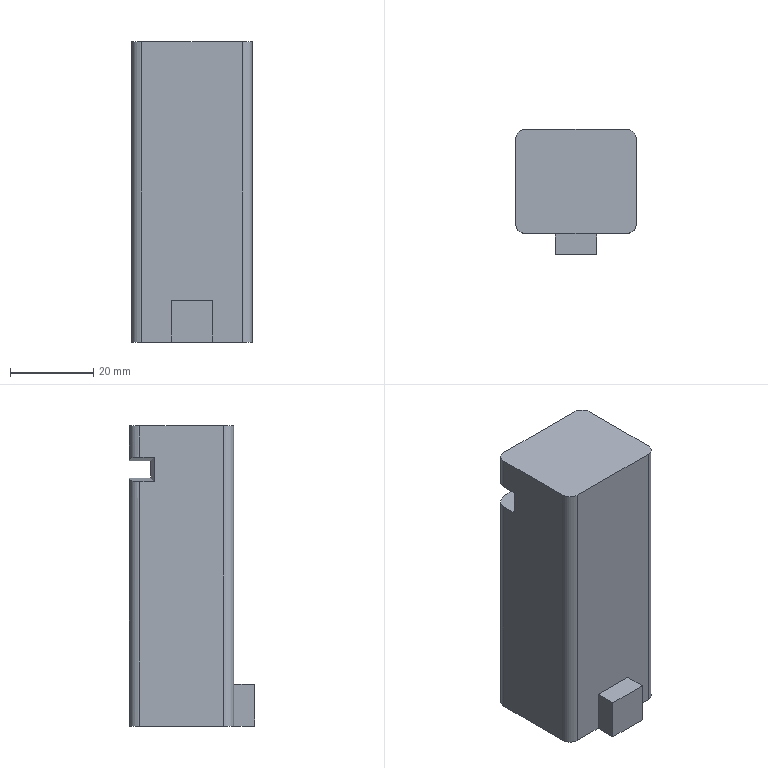Part | NX | features 1605340631 2 | 1 solid | 28 faces | box 29 x 30 x 72 mm | volume 45526 mm3 | plane 21 | cylinder 7 | commonest cylinder face diameters 5 x6 17 x1
STEP:
#1=CARTESIAN_POINT('',(-139.5,-95.3,2.1));
#2=VERTEX_POINT('',#1);
#3=CARTESIAN_POINT('',(-120.5,-95.3,2.1));
#4=VERTEX_POINT('',#3);
#5=CARTESIAN_POINT('',(-131.872,-95.3,2.1));
#6=DIRECTION('',(1.,0.,0.));
#7=VECTOR('',#6,1000.);
#8=LINE('',#5,#7);
#9=EDGE_CURVE('',#2,#4,#8,.T.);
#10=ORIENTED_EDGE('',*,*,#9,.T.);
#11=CARTESIAN_POINT('',(-120.5,-95.3,-2.));
#12=VERTEX_POINT('',#11);
#13=CARTESIAN_POINT('',(-120.5,-95.3,-0.1));
#14=DIRECTION('',(0.,0.,-1.));
#15=VECTOR('',#14,1000.);
#16=LINE('',#13,#15);
#17=EDGE_CURVE('',#4,#12,#16,.T.);
#18=ORIENTED_EDGE('',*,*,#17,.T.);
#19=CARTESIAN_POINT('',(-139.5,-95.3,-2.));
#20=VERTEX_POINT('',#19);
#21=CARTESIAN_POINT('',(165.,-95.3,-2.));
#22=DIRECTION('',(-1.,0.,0.));
#23=VECTOR('',#22,1000.);
#24=LINE('',#21,#23);
#25=EDGE_CURVE('',#12,#20,#24,.T.);
#26=ORIENTED_EDGE('',*,*,#25,.T.);
#27=CARTESIAN_POINT('',(-139.5,-95.3,-0.1));
#28=DIRECTION('',(0.,0.,1.));
#29=VECTOR('',#28,1000.);
#30=LINE('',#27,#29);
#31=EDGE_CURVE('',#20,#2,#30,.T.);
#32=ORIENTED_EDGE('',*,*,#31,.T.);
#33=EDGE_LOOP('',(#10,#18,#26,#32));
#34=FACE_BOUND('',#33,.T.);
#35=CARTESIAN_POINT('',(-131.872,-95.3,-0.1));
#36=DIRECTION('',(0.,1.,0.));
#37=DIRECTION('',(-1.,0.,0.));
#38=AXIS2_PLACEMENT_3D('',#35,#36,#37);
#39=PLANE('',#38);
#40=ADVANCED_FACE('',(#34),#39,.T.);
#41=ORIENTED_EDGE('',*,*,#25,.F.);
#42=CARTESIAN_POINT('',(-120.5,-90.2,-2.));
#43=VERTEX_POINT('',#42);
#44=CARTESIAN_POINT('',(-120.5,-31.936,-2.));
#45=DIRECTION('',(0.,1.,0.));
#46=VECTOR('',#45,1000.);
#47=LINE('',#44,#46);
#48=EDGE_CURVE('',#12,#43,#47,.T.);
#49=ORIENTED_EDGE('',*,*,#48,.T.);
#50=CARTESIAN_POINT('',(-139.5,-90.2,-2.));
#51=VERTEX_POINT('',#50);
#52=CARTESIAN_POINT('',(165.,-90.2,-2.));
#53=DIRECTION('',(-1.,0.,0.));
#54=VECTOR('',#53,1000.);
#55=LINE('',#52,#54);
#56=EDGE_CURVE('',#43,#51,#55,.T.);
#57=ORIENTED_EDGE('',*,*,#56,.T.);
#58=CARTESIAN_POINT('',(-139.5,-31.936,-2.));
#59=DIRECTION('',(0.,-1.,0.));
#60=VECTOR('',#59,1000.);
#61=LINE('',#58,#60);
#62=EDGE_CURVE('',#51,#20,#61,.T.);
#63=ORIENTED_EDGE('',*,*,#62,.T.);
#64=EDGE_LOOP('',(#41,#49,#57,#63));
#65=FACE_BOUND('',#64,.T.);
#66=CARTESIAN_POINT('',(165.,-31.936,-2.));
#67=DIRECTION('',(0.,0.,1.));
#68=DIRECTION('',(1.,0.,0.));
#69=AXIS2_PLACEMENT_3D('',#66,#67,#68);
#70=PLANE('',#69);
#71=ADVANCED_FACE('',(#65),#70,.T.);
#72=ORIENTED_EDGE('',*,*,#56,.F.);
#73=CARTESIAN_POINT('',(-118.,-90.2,-2.441));
#74=VERTEX_POINT('',#73);
#75=CARTESIAN_POINT('',(-133.512,-90.2,0.2944));
#76=DIRECTION('',(-0.9848,0.,0.1736));
#77=VECTOR('',#76,1000.);
#78=LINE('',#75,#77);
#79=EDGE_CURVE('',#43,#74,#78,.F.);
#80=ORIENTED_EDGE('',*,*,#79,.T.);
#81=CARTESIAN_POINT('',(-118.,-90.2,-61.5));
#82=VERTEX_POINT('',#81);
#83=CARTESIAN_POINT('',(-118.,-90.2,-36.501));
#84=DIRECTION('',(0.,0.,-1.));
#85=VECTOR('',#84,1000.);
#86=LINE('',#83,#85);
#87=EDGE_CURVE('',#74,#82,#86,.T.);
#88=ORIENTED_EDGE('',*,*,#87,.T.);
#89=CARTESIAN_POINT('',(-142.,-90.2,-61.5));
#90=VERTEX_POINT('',#89);
#91=CARTESIAN_POINT('',(-180.,-90.2,-61.5));
#92=DIRECTION('',(1.,0.,0.));
#93=VECTOR('',#92,1000.);
#94=LINE('',#91,#93);
#95=EDGE_CURVE('',#90,#82,#94,.T.);
#96=ORIENTED_EDGE('',*,*,#95,.F.);
#97=CARTESIAN_POINT('',(-142.,-90.2,-2.441));
#98=VERTEX_POINT('',#97);
#99=CARTESIAN_POINT('',(-142.,-90.2,-36.501));
#100=DIRECTION('',(0.,0.,-1.));
#101=VECTOR('',#100,1000.);
#102=LINE('',#99,#101);
#103=EDGE_CURVE('',#90,#98,#102,.F.);
#104=ORIENTED_EDGE('',*,*,#103,.T.);
#105=CARTESIAN_POINT('',(-145.885,-90.2,-3.126));
#106=DIRECTION('',(-0.9848,0.,-0.1736));
#107=VECTOR('',#106,1000.);
#108=LINE('',#105,#107);
#109=EDGE_CURVE('',#98,#51,#108,.F.);
#110=ORIENTED_EDGE('',*,*,#109,.T.);
#111=EDGE_LOOP('',(#72,#80,#88,#96,#104,#110));
#112=FACE_BOUND('',#111,.T.);
#113=CARTESIAN_POINT('',(-140.,-90.2,-36.501));
#114=DIRECTION('',(0.,1.,0.));
#115=DIRECTION('',(0.,0.,1.));
#116=AXIS2_PLACEMENT_3D('',#113,#114,#115);
#117=PLANE('',#116);
#118=ADVANCED_FACE('',(#112),#117,.T.);
#119=CARTESIAN_POINT('',(-139.5,-90.2,2.1));
#120=VERTEX_POINT('',#119);
#121=CARTESIAN_POINT('',(-120.5,-90.2,2.1));
#122=VERTEX_POINT('',#121);
#123=CARTESIAN_POINT('',(-140.,-90.2,2.1));
#124=DIRECTION('',(1.,0.,0.));
#125=VECTOR('',#124,1000.);
#126=LINE('',#123,#125);
#127=EDGE_CURVE('',#120,#122,#126,.T.);
#128=ORIENTED_EDGE('',*,*,#127,.T.);
#129=CARTESIAN_POINT('',(-120.5,-95.3,2.1));
#130=DIRECTION('',(0.,-1.,0.));
#131=VECTOR('',#130,1000.);
#132=LINE('',#129,#131);
#133=EDGE_CURVE('',#122,#4,#132,.T.);
#134=ORIENTED_EDGE('',*,*,#133,.T.);
#135=ORIENTED_EDGE('',*,*,#9,.F.);
#136=CARTESIAN_POINT('',(-139.5,-92.2,2.1));
#137=DIRECTION('',(0.,1.,0.));
#138=VECTOR('',#137,1000.);
#139=LINE('',#136,#138);
#140=EDGE_CURVE('',#2,#120,#139,.T.);
#141=ORIENTED_EDGE('',*,*,#140,.T.);
#142=EDGE_LOOP('',(#128,#134,#135,#141));
#143=FACE_BOUND('',#142,.T.);
#144=CARTESIAN_POINT('',(-140.,-110.2,2.1));
#145=DIRECTION('',(0.,0.,1.));
#146=DIRECTION('',(1.,0.,0.));
#147=AXIS2_PLACEMENT_3D('',#144,#145,#146);
#148=PLANE('',#147);
#149=ADVANCED_FACE('',(#143),#148,.F.);
#150=CARTESIAN_POINT('',(-118.,-90.2,10.5));
#151=VERTEX_POINT('',#150);
#152=CARTESIAN_POINT('',(-118.,-90.2,2.541));
#153=VERTEX_POINT('',#152);
#154=CARTESIAN_POINT('',(-118.,-90.2,-37.901));
#155=DIRECTION('',(0.,0.,1.));
#156=VECTOR('',#155,1000.);
#157=LINE('',#154,#156);
#158=EDGE_CURVE('',#151,#153,#157,.F.);
#159=ORIENTED_EDGE('',*,*,#158,.T.);
#160=CARTESIAN_POINT('',(-146.253,-90.2,-2.441));
#161=DIRECTION('',(-0.9848,0.,-0.1736));
#162=VECTOR('',#161,1000.);
#163=LINE('',#160,#162);
#164=EDGE_CURVE('',#153,#122,#163,.T.);
#165=ORIENTED_EDGE('',*,*,#164,.T.);
#166=ORIENTED_EDGE('',*,*,#127,.F.);
#167=CARTESIAN_POINT('',(-142.,-90.2,2.541));
#168=VERTEX_POINT('',#167);
#169=CARTESIAN_POINT('',(-133.144,-90.2,0.9793));
#170=DIRECTION('',(-0.9848,0.,0.1736));
#171=VECTOR('',#170,1000.);
#172=LINE('',#169,#171);
#173=EDGE_CURVE('',#120,#168,#172,.T.);
#174=ORIENTED_EDGE('',*,*,#173,.T.);
#175=CARTESIAN_POINT('',(-142.,-90.2,10.5));
#176=VERTEX_POINT('',#175);
#177=CARTESIAN_POINT('',(-142.,-90.2,-37.901));
#178=DIRECTION('',(0.,0.,1.));
#179=VECTOR('',#178,1000.);
#180=LINE('',#177,#179);
#181=EDGE_CURVE('',#168,#176,#180,.T.);
#182=ORIENTED_EDGE('',*,*,#181,.T.);
#183=CARTESIAN_POINT('',(-140.,-90.2,10.5));
#184=DIRECTION('',(-1.,0.,0.));
#185=VECTOR('',#184,1000.);
#186=LINE('',#183,#185);
#187=EDGE_CURVE('',#151,#176,#186,.T.);
#188=ORIENTED_EDGE('',*,*,#187,.F.);
#189=EDGE_LOOP('',(#159,#165,#166,#174,#182,#188));
#190=FACE_BOUND('',#189,.T.);
#191=CARTESIAN_POINT('',(-140.,-90.2,-37.901));
#192=DIRECTION('',(0.,1.,0.));
#193=DIRECTION('',(0.,0.,1.));
#194=AXIS2_PLACEMENT_3D('',#191,#192,#193);
#195=PLANE('',#194);
#196=ADVANCED_FACE('',(#190),#195,.T.);
#197=CARTESIAN_POINT('',(-142.,-115.2,10.5));
#198=VERTEX_POINT('',#197);
#199=CARTESIAN_POINT('',(-118.,-115.2,10.5));
#200=VERTEX_POINT('',#199);
#201=CARTESIAN_POINT('',(-120.,-115.2,10.5));
#202=DIRECTION('',(1.,0.,0.));
#203=VECTOR('',#202,1000.);
#204=LINE('',#201,#203);
#205=EDGE_CURVE('',#198,#200,#204,.T.);
#206=ORIENTED_EDGE('',*,*,#205,.F.);
#207=CARTESIAN_POINT('',(-142.,-115.2,-61.5));
#208=VERTEX_POINT('',#207);
#209=CARTESIAN_POINT('',(-142.,-115.2,-36.501));
#210=DIRECTION('',(0.,0.,-1.));
#211=VECTOR('',#210,1000.);
#212=LINE('',#209,#211);
#213=EDGE_CURVE('',#198,#208,#212,.T.);
#214=ORIENTED_EDGE('',*,*,#213,.T.);
#215=CARTESIAN_POINT('',(-135.,-115.2,-61.5));
#216=VERTEX_POINT('',#215);
#217=CARTESIAN_POINT('',(-180.,-115.2,-61.5));
#218=DIRECTION('',(-1.,0.,0.));
#219=VECTOR('',#218,1000.);
#220=LINE('',#217,#219);
#221=EDGE_CURVE('',#216,#208,#220,.T.);
#222=ORIENTED_EDGE('',*,*,#221,.F.);
#223=CARTESIAN_POINT('',(-135.,-115.2,-51.5));
#224=VERTEX_POINT('',#223);
#225=CARTESIAN_POINT('',(-135.,-115.2,-26.501));
#226=DIRECTION('',(0.,0.,-1.));
#227=VECTOR('',#226,1000.);
#228=LINE('',#225,#227);
#229=EDGE_CURVE('',#224,#216,#228,.T.);
#230=ORIENTED_EDGE('',*,*,#229,.F.);
#231=CARTESIAN_POINT('',(-125.,-115.2,-51.5));
#232=VERTEX_POINT('',#231);
#233=CARTESIAN_POINT('',(-120.,-115.2,-51.5));
#234=DIRECTION('',(1.,0.,0.));
#235=VECTOR('',#234,1000.);
#236=LINE('',#233,#235);
#237=EDGE_CURVE('',#224,#232,#236,.T.);
#238=ORIENTED_EDGE('',*,*,#237,.T.);
#239=CARTESIAN_POINT('',(-125.,-115.2,-61.5));
#240=VERTEX_POINT('',#239);
#241=CARTESIAN_POINT('',(-125.,-115.2,-26.501));
#242=DIRECTION('',(0.,0.,-1.));
#243=VECTOR('',#242,1000.);
#244=LINE('',#241,#243);
#245=EDGE_CURVE('',#232,#240,#244,.T.);
#246=ORIENTED_EDGE('',*,*,#245,.T.);
#247=CARTESIAN_POINT('',(-118.,-115.2,-61.5));
#248=VERTEX_POINT('',#247);
#249=CARTESIAN_POINT('',(-180.,-115.2,-61.5));
#250=DIRECTION('',(-1.,0.,0.));
#251=VECTOR('',#250,1000.);
#252=LINE('',#249,#251);
#253=EDGE_CURVE('',#248,#240,#252,.T.);
#254=ORIENTED_EDGE('',*,*,#253,.F.);
#255=CARTESIAN_POINT('',(-118.,-115.2,-36.501));
#256=DIRECTION('',(0.,0.,-1.));
#257=VECTOR('',#256,1000.);
#258=LINE('',#255,#257);
#259=EDGE_CURVE('',#248,#200,#258,.F.);
#260=ORIENTED_EDGE('',*,*,#259,.T.);
#261=EDGE_LOOP('',(#206,#214,#222,#230,#238,#246,#254,#260));
#262=FACE_BOUND('',#261,.T.);
#263=CARTESIAN_POINT('',(-120.,-115.2,-36.501));
#264=DIRECTION('',(0.,-1.,0.));
#265=DIRECTION('',(0.,0.,-1.));
#266=AXIS2_PLACEMENT_3D('',#263,#264,#265);
#267=PLANE('',#266);
#268=ADVANCED_FACE('',(#262),#267,.T.);
#269=CARTESIAN_POINT('',(-138.5,-102.7,-61.5));
#270=VERTEX_POINT('',#269);
#271=CARTESIAN_POINT('',(-130.,-102.7,-61.5));
#272=DIRECTION('',(0.,0.,-1.));
#273=DIRECTION('',(-1.,0.,0.));
#274=AXIS2_PLACEMENT_3D('',#271,#272,#273);
#275=CIRCLE('',#274,8.5);
#276=EDGE_CURVE('',#270,#270,#275,.F.);
#277=ORIENTED_EDGE('',*,*,#276,.T.);
#278=EDGE_LOOP('',(#277));
#279=FACE_BOUND('',#278,.T.);
#280=ORIENTED_EDGE('',*,*,#253,.T.);
#281=CARTESIAN_POINT('',(-125.,-120.2,-61.5));
#282=VERTEX_POINT('',#281);
#283=CARTESIAN_POINT('',(-125.,-167.2,-61.5));
#284=DIRECTION('',(0.,1.,0.));
#285=VECTOR('',#284,1000.);
#286=LINE('',#283,#285);
#287=EDGE_CURVE('',#282,#240,#286,.T.);
#288=ORIENTED_EDGE('',*,*,#287,.F.);
#289=CARTESIAN_POINT('',(-135.,-120.2,-61.5));
#290=VERTEX_POINT('',#289);
#291=CARTESIAN_POINT('',(-180.,-120.2,-61.5));
#292=DIRECTION('',(-1.,0.,0.));
#293=VECTOR('',#292,1000.);
#294=LINE('',#291,#293);
#295=EDGE_CURVE('',#282,#290,#294,.T.);
#296=ORIENTED_EDGE('',*,*,#295,.T.);
#297=CARTESIAN_POINT('',(-135.,-167.2,-61.5));
#298=DIRECTION('',(0.,1.,0.));
#299=VECTOR('',#298,1000.);
#300=LINE('',#297,#299);
#301=EDGE_CURVE('',#290,#216,#300,.T.);
#302=ORIENTED_EDGE('',*,*,#301,.T.);
#303=ORIENTED_EDGE('',*,*,#221,.T.);
#304=CARTESIAN_POINT('',(-144.5,-112.7,-61.5));
#305=VERTEX_POINT('',#304);
#306=CARTESIAN_POINT('',(-142.,-112.7,-61.5));
#307=DIRECTION('',(0.,0.,-1.));
#308=DIRECTION('',(-1.,0.,0.));
#309=AXIS2_PLACEMENT_3D('',#306,#307,#308);
#310=CIRCLE('',#309,2.5);
#311=EDGE_CURVE('',#208,#305,#310,.T.);
#312=ORIENTED_EDGE('',*,*,#311,.T.);
#313=CARTESIAN_POINT('',(-144.5,-92.7,-61.5));
#314=VERTEX_POINT('',#313);
#315=CARTESIAN_POINT('',(-144.5,-167.2,-61.5));
#316=DIRECTION('',(0.,1.,0.));
#317=VECTOR('',#316,1000.);
#318=LINE('',#315,#317);
#319=EDGE_CURVE('',#305,#314,#318,.T.);
#320=ORIENTED_EDGE('',*,*,#319,.T.);
#321=CARTESIAN_POINT('',(-142.,-92.7,-61.5));
#322=DIRECTION('',(0.,0.,-1.));
#323=DIRECTION('',(-1.,0.,0.));
#324=AXIS2_PLACEMENT_3D('',#321,#322,#323);
#325=CIRCLE('',#324,2.5);
#326=EDGE_CURVE('',#314,#90,#325,.T.);
#327=ORIENTED_EDGE('',*,*,#326,.T.);
#328=ORIENTED_EDGE('',*,*,#95,.T.);
#329=CARTESIAN_POINT('',(-115.5,-92.7,-61.5));
#330=VERTEX_POINT('',#329);
#331=CARTESIAN_POINT('',(-118.,-92.7,-61.5));
#332=DIRECTION('',(0.,0.,-1.));
#333=DIRECTION('',(-1.,0.,0.));
#334=AXIS2_PLACEMENT_3D('',#331,#332,#333);
#335=CIRCLE('',#334,2.5);
#336=EDGE_CURVE('',#82,#330,#335,.T.);
#337=ORIENTED_EDGE('',*,*,#336,.T.);
#338=CARTESIAN_POINT('',(-115.5,-112.7,-61.5));
#339=VERTEX_POINT('',#338);
#340=CARTESIAN_POINT('',(-115.5,-167.2,-61.5));
#341=DIRECTION('',(0.,-1.,0.));
#342=VECTOR('',#341,1000.);
#343=LINE('',#340,#342);
#344=EDGE_CURVE('',#330,#339,#343,.T.);
#345=ORIENTED_EDGE('',*,*,#344,.T.);
#346=CARTESIAN_POINT('',(-118.,-112.7,-61.5));
#347=DIRECTION('',(0.,0.,-1.));
#348=DIRECTION('',(-1.,0.,0.));
#349=AXIS2_PLACEMENT_3D('',#346,#347,#348);
#350=CIRCLE('',#349,2.5);
#351=EDGE_CURVE('',#339,#248,#350,.T.);
#352=ORIENTED_EDGE('',*,*,#351,.T.);
#353=EDGE_LOOP('',(#280,#288,#296,#302,#303,#312,#320,#327,#328,#337,#345,#352));
#354=FACE_BOUND('',#353,.T.);
#355=CARTESIAN_POINT('',(-180.,-167.2,-61.5));
#356=DIRECTION('',(0.,0.,-1.));
#357=DIRECTION('',(-1.,0.,0.));
#358=AXIS2_PLACEMENT_3D('',#355,#356,#357);
#359=PLANE('',#358);
#360=ADVANCED_FACE('',(#279,#354),#359,.T.);
#361=ORIENTED_EDGE('',*,*,#87,.F.);
#362=CARTESIAN_POINT('',(-115.5,-92.7,-2.882));
#363=VERTEX_POINT('',#362);
#364=CARTESIAN_POINT('',(-118.,-92.7,-2.441));
#365=DIRECTION('',(-0.1736,0.,-0.9848));
#366=DIRECTION('',(0.9848,0.,-0.1736));
#367=AXIS2_PLACEMENT_3D('',#364,#365,#366);
#368=ELLIPSE('',#367,2.539,2.5);
#369=EDGE_CURVE('',#74,#363,#368,.T.);
#370=ORIENTED_EDGE('',*,*,#369,.T.);
#371=CARTESIAN_POINT('',(-115.5,-92.7,-36.501));
#372=DIRECTION('',(0.,0.,-1.));
#373=VECTOR('',#372,1000.);
#374=LINE('',#371,#373);
#375=EDGE_CURVE('',#330,#363,#374,.F.);
#376=ORIENTED_EDGE('',*,*,#375,.F.);
#377=ORIENTED_EDGE('',*,*,#336,.F.);
#378=EDGE_LOOP('',(#361,#370,#376,#377));
#379=FACE_BOUND('',#378,.T.);
#380=CARTESIAN_POINT('',(-118.,-92.7,-36.501));
#381=DIRECTION('',(0.,0.,-1.));
#382=DIRECTION('',(-1.,0.,0.));
#383=AXIS2_PLACEMENT_3D('',#380,#381,#382);
#384=CYLINDRICAL_SURFACE('',#383,2.5);
#385=ADVANCED_FACE('',(#379),#384,.T.);
#386=ORIENTED_EDGE('',*,*,#351,.F.);
#387=CARTESIAN_POINT('',(-115.5,-112.7,10.5));
#388=VERTEX_POINT('',#387);
#389=CARTESIAN_POINT('',(-115.5,-112.7,-36.501));
#390=DIRECTION('',(0.,0.,-1.));
#391=VECTOR('',#390,1000.);
#392=LINE('',#389,#391);
#393=EDGE_CURVE('',#388,#339,#392,.T.);
#394=ORIENTED_EDGE('',*,*,#393,.F.);
#395=CARTESIAN_POINT('',(-118.,-112.7,10.5));
#396=DIRECTION('',(0.,0.,1.));
#397=DIRECTION('',(1.,0.,0.));
#398=AXIS2_PLACEMENT_3D('',#395,#396,#397);
#399=CIRCLE('',#398,2.5);
#400=EDGE_CURVE('',#200,#388,#399,.T.);
#401=ORIENTED_EDGE('',*,*,#400,.F.);
#402=ORIENTED_EDGE('',*,*,#259,.F.);
#403=EDGE_LOOP('',(#386,#394,#401,#402));
#404=FACE_BOUND('',#403,.T.);
#405=CARTESIAN_POINT('',(-118.,-112.7,-36.501));
#406=DIRECTION('',(0.,0.,-1.));
#407=DIRECTION('',(-1.,0.,0.));
#408=AXIS2_PLACEMENT_3D('',#405,#406,#407);
#409=CYLINDRICAL_SURFACE('',#408,2.5);
#410=ADVANCED_FACE('',(#404),#409,.T.);
#411=CARTESIAN_POINT('',(-115.5,-96.182,-2.882));
#412=VERTEX_POINT('',#411);
#413=CARTESIAN_POINT('',(-115.5,-96.182,2.982));
#414=VERTEX_POINT('',#413);
#415=CARTESIAN_POINT('',(-115.5,-96.182,-36.501));
#416=DIRECTION('',(0.,0.,1.));
#417=VECTOR('',#416,1000.);
#418=LINE('',#415,#417);
#419=EDGE_CURVE('',#412,#414,#418,.T.);
#420=ORIENTED_EDGE('',*,*,#419,.T.);
#421=CARTESIAN_POINT('',(-115.5,-92.7,2.982));
#422=VERTEX_POINT('',#421);
#423=CARTESIAN_POINT('',(-115.5,-92.2,2.982));
#424=DIRECTION('',(0.,1.,0.));
#425=VECTOR('',#424,1000.);
#426=LINE('',#423,#425);
#427=EDGE_CURVE('',#414,#422,#426,.T.);
#428=ORIENTED_EDGE('',*,*,#427,.T.);
#429=CARTESIAN_POINT('',(-115.5,-92.7,10.5));
#430=VERTEX_POINT('',#429);
#431=CARTESIAN_POINT('',(-115.5,-92.7,-36.501));
#432=DIRECTION('',(0.,0.,1.));
#433=VECTOR('',#432,1000.);
#434=LINE('',#431,#433);
#435=EDGE_CURVE('',#422,#430,#434,.T.);
#436=ORIENTED_EDGE('',*,*,#435,.T.);
#437=CARTESIAN_POINT('',(-115.5,-90.2,10.5));
#438=DIRECTION('',(0.,1.,0.));
#439=VECTOR('',#438,1000.);
#440=LINE('',#437,#439);
#441=EDGE_CURVE('',#388,#430,#440,.T.);
#442=ORIENTED_EDGE('',*,*,#441,.F.);
#443=ORIENTED_EDGE('',*,*,#393,.T.);
#444=ORIENTED_EDGE('',*,*,#344,.F.);
#445=ORIENTED_EDGE('',*,*,#375,.T.);
#446=CARTESIAN_POINT('',(-115.5,-90.2,-2.882));
#447=DIRECTION('',(0.,-1.,0.));
#448=VECTOR('',#447,1000.);
#449=LINE('',#446,#448);
#450=EDGE_CURVE('',#363,#412,#449,.T.);
#451=ORIENTED_EDGE('',*,*,#450,.T.);
#452=EDGE_LOOP('',(#420,#428,#436,#442,#443,#444,#445,#451));
#453=FACE_BOUND('',#452,.T.);
#454=CARTESIAN_POINT('',(-115.5,-90.2,-36.501));
#455=DIRECTION('',(1.,0.,0.));
#456=DIRECTION('',(0.,0.,-1.));
#457=AXIS2_PLACEMENT_3D('',#454,#455,#456);
#458=PLANE('',#457);
#459=ADVANCED_FACE('',(#453),#458,.T.);
#460=ORIENTED_EDGE('',*,*,#435,.F.);
#461=CARTESIAN_POINT('',(-118.,-92.7,2.541));
#462=DIRECTION('',(0.1736,0.,-0.9848));
#463=DIRECTION('',(0.9848,0.,0.1736));
#464=AXIS2_PLACEMENT_3D('',#461,#462,#463);
#465=ELLIPSE('',#464,2.539,2.5);
#466=EDGE_CURVE('',#422,#153,#465,.F.);
#467=ORIENTED_EDGE('',*,*,#466,.T.);
#468=ORIENTED_EDGE('',*,*,#158,.F.);
#469=CARTESIAN_POINT('',(-118.,-92.7,10.5));
#470=DIRECTION('',(0.,0.,1.));
#471=DIRECTION('',(1.,0.,0.));
#472=AXIS2_PLACEMENT_3D('',#469,#470,#471);
#473=CIRCLE('',#472,2.5);
#474=EDGE_CURVE('',#430,#151,#473,.T.);
#475=ORIENTED_EDGE('',*,*,#474,.F.);
#476=EDGE_LOOP('',(#460,#467,#468,#475));
#477=FACE_BOUND('',#476,.T.);
#478=CARTESIAN_POINT('',(-118.,-92.7,-36.501));
#479=DIRECTION('',(0.,0.,1.));
#480=DIRECTION('',(1.,0.,0.));
#481=AXIS2_PLACEMENT_3D('',#478,#479,#480);
#482=CYLINDRICAL_SURFACE('',#481,2.5);
#483=ADVANCED_FACE('',(#477),#482,.T.);
#484=CARTESIAN_POINT('',(-144.5,-92.7,10.5));
#485=VERTEX_POINT('',#484);
#486=CARTESIAN_POINT('',(-144.5,-92.7,2.982));
#487=VERTEX_POINT('',#486);
#488=CARTESIAN_POINT('',(-144.5,-92.7,-36.501));
#489=DIRECTION('',(0.,0.,1.));
#490=VECTOR('',#489,1000.);
#491=LINE('',#488,#490);
#492=EDGE_CURVE('',#485,#487,#491,.F.);
#493=ORIENTED_EDGE('',*,*,#492,.T.);
#494=CARTESIAN_POINT('',(-144.5,-96.182,2.982));
#495=VERTEX_POINT('',#494);
#496=CARTESIAN_POINT('',(-144.5,-95.3,2.982));
#497=DIRECTION('',(0.,-1.,0.));
#498=VECTOR('',#497,1000.);
#499=LINE('',#496,#498);
#500=EDGE_CURVE('',#487,#495,#499,.T.);
#501=ORIENTED_EDGE('',*,*,#500,.T.);
#502=CARTESIAN_POINT('',(-144.5,-96.182,-2.882));
#503=VERTEX_POINT('',#502);
#504=CARTESIAN_POINT('',(-144.5,-96.182,-36.501));
#505=DIRECTION('',(0.,0.,-1.));
#506=VECTOR('',#505,1000.);
#507=LINE('',#504,#506);
#508=EDGE_CURVE('',#495,#503,#507,.T.);
#509=ORIENTED_EDGE('',*,*,#508,.T.);
#510=CARTESIAN_POINT('',(-144.5,-92.7,-2.882));
#511=VERTEX_POINT('',#510);
#512=CARTESIAN_POINT('',(-144.5,-110.2,-2.882));
#513=DIRECTION('',(0.,1.,0.));
#514=VECTOR('',#513,1000.);
#515=LINE('',#512,#514);
#516=EDGE_CURVE('',#503,#511,#515,.T.);
#517=ORIENTED_EDGE('',*,*,#516,.T.);
#518=CARTESIAN_POINT('',(-144.5,-92.7,-36.501));
#519=DIRECTION('',(0.,0.,-1.));
#520=VECTOR('',#519,1000.);
#521=LINE('',#518,#520);
#522=EDGE_CURVE('',#511,#314,#521,.T.);
#523=ORIENTED_EDGE('',*,*,#522,.T.);
#524=ORIENTED_EDGE('',*,*,#319,.F.);
#525=CARTESIAN_POINT('',(-144.5,-112.7,10.5));
#526=VERTEX_POINT('',#525);
#527=CARTESIAN_POINT('',(-144.5,-112.7,-36.501));
#528=DIRECTION('',(0.,0.,-1.));
#529=VECTOR('',#528,1000.);
#530=LINE('',#527,#529);
#531=EDGE_CURVE('',#305,#526,#530,.F.);
#532=ORIENTED_EDGE('',*,*,#531,.T.);
#533=CARTESIAN_POINT('',(-144.5,-110.2,10.5));
#534=DIRECTION('',(0.,-1.,0.));
#535=VECTOR('',#534,1000.);
#536=LINE('',#533,#535);
#537=EDGE_CURVE('',#485,#526,#536,.T.);
#538=ORIENTED_EDGE('',*,*,#537,.F.);
#539=EDGE_LOOP('',(#493,#501,#509,#517,#523,#524,#532,#538));
#540=FACE_BOUND('',#539,.T.);
#541=CARTESIAN_POINT('',(-144.5,-110.2,-36.501));
#542=DIRECTION('',(-1.,0.,0.));
#543=DIRECTION('',(0.,0.,1.));
#544=AXIS2_PLACEMENT_3D('',#541,#542,#543);
#545=PLANE('',#544);
#546=ADVANCED_FACE('',(#540),#545,.T.);
#547=ORIENTED_EDGE('',*,*,#311,.F.);
#548=ORIENTED_EDGE('',*,*,#213,.F.);
#549=CARTESIAN_POINT('',(-142.,-112.7,10.5));
#550=DIRECTION('',(0.,0.,1.));
#551=DIRECTION('',(1.,0.,0.));
#552=AXIS2_PLACEMENT_3D('',#549,#550,#551);
#553=CIRCLE('',#552,2.5);
#554=EDGE_CURVE('',#526,#198,#553,.T.);
#555=ORIENTED_EDGE('',*,*,#554,.F.);
#556=ORIENTED_EDGE('',*,*,#531,.F.);
#557=EDGE_LOOP('',(#547,#548,#555,#556));
#558=FACE_BOUND('',#557,.T.);
#559=CARTESIAN_POINT('',(-142.,-112.7,-36.501));
#560=DIRECTION('',(0.,0.,-1.));
#561=DIRECTION('',(-1.,0.,0.));
#562=AXIS2_PLACEMENT_3D('',#559,#560,#561);
#563=CYLINDRICAL_SURFACE('',#562,2.5);
#564=ADVANCED_FACE('',(#558),#563,.T.);
#565=ORIENTED_EDGE('',*,*,#522,.F.);
#566=CARTESIAN_POINT('',(-142.,-92.7,-2.441));
#567=DIRECTION('',(0.1736,0.,-0.9848));
#568=DIRECTION('',(-0.9848,0.,-0.1736));
#569=AXIS2_PLACEMENT_3D('',#566,#567,#568);
#570=ELLIPSE('',#569,2.539,2.5);
#571=EDGE_CURVE('',#511,#98,#570,.T.);
#572=ORIENTED_EDGE('',*,*,#571,.T.);
#573=ORIENTED_EDGE('',*,*,#103,.F.);
#574=ORIENTED_EDGE('',*,*,#326,.F.);
#575=EDGE_LOOP('',(#565,#572,#573,#574));
#576=FACE_BOUND('',#575,.T.);
#577=CARTESIAN_POINT('',(-142.,-92.7,-36.501));
#578=DIRECTION('',(0.,0.,-1.));
#579=DIRECTION('',(-1.,0.,0.));
#580=AXIS2_PLACEMENT_3D('',#577,#578,#579);
#581=CYLINDRICAL_SURFACE('',#580,2.5);
#582=ADVANCED_FACE('',(#576),#581,.T.);
#583=ORIENTED_EDGE('',*,*,#181,.F.);
#584=CARTESIAN_POINT('',(-142.,-92.7,2.541));
#585=DIRECTION('',(-0.1736,0.,-0.9848));
#586=DIRECTION('',(-0.9848,0.,0.1736));
#587=AXIS2_PLACEMENT_3D('',#584,#585,#586);
#588=ELLIPSE('',#587,2.539,2.5);
#589=EDGE_CURVE('',#168,#487,#588,.F.);
#590=ORIENTED_EDGE('',*,*,#589,.T.);
#591=ORIENTED_EDGE('',*,*,#492,.F.);
#592=CARTESIAN_POINT('',(-142.,-92.7,10.5));
#593=DIRECTION('',(0.,0.,1.));
#594=DIRECTION('',(1.,0.,0.));
#595=AXIS2_PLACEMENT_3D('',#592,#593,#594);
#596=CIRCLE('',#595,2.5);
#597=EDGE_CURVE('',#176,#485,#596,.T.);
#598=ORIENTED_EDGE('',*,*,#597,.F.);
#599=EDGE_LOOP('',(#583,#590,#591,#598));
#600=FACE_BOUND('',#599,.T.);
#601=CARTESIAN_POINT('',(-142.,-92.7,-37.901));
#602=DIRECTION('',(0.,0.,1.));
#603=DIRECTION('',(1.,0.,0.));
#604=AXIS2_PLACEMENT_3D('',#601,#602,#603);
#605=CYLINDRICAL_SURFACE('',#604,2.5);
#606=ADVANCED_FACE('',(#600),#605,.T.);
#607=ORIENTED_EDGE('',*,*,#245,.F.);
#608=CARTESIAN_POINT('',(-125.,-120.2,-51.5));
#609=VERTEX_POINT('',#608);
#610=CARTESIAN_POINT('',(-125.,-115.2,-51.5));
#611=DIRECTION('',(0.,-1.,0.));
#612=VECTOR('',#611,1000.);
#613=LINE('',#610,#612);
#614=EDGE_CURVE('',#232,#609,#613,.T.);
#615=ORIENTED_EDGE('',*,*,#614,.T.);
#616=CARTESIAN_POINT('',(-125.,-120.2,-26.501));
#617=DIRECTION('',(0.,0.,-1.));
#618=VECTOR('',#617,1000.);
#619=LINE('',#616,#618);
#620=EDGE_CURVE('',#609,#282,#619,.T.);
#621=ORIENTED_EDGE('',*,*,#620,.T.);
#622=ORIENTED_EDGE('',*,*,#287,.T.);
#623=EDGE_LOOP('',(#607,#615,#621,#622));
#624=FACE_BOUND('',#623,.T.);
#625=CARTESIAN_POINT('',(-125.,-115.2,-61.5));
#626=DIRECTION('',(-1.,0.,0.));
#627=DIRECTION('',(0.,-1.,0.));
#628=AXIS2_PLACEMENT_3D('',#625,#626,#627);
#629=PLANE('',#628);
#630=ADVANCED_FACE('',(#624),#629,.F.);
#631=CARTESIAN_POINT('',(-135.,-120.2,-51.5));
#632=VERTEX_POINT('',#631);
#633=CARTESIAN_POINT('',(-120.,-120.2,-51.5));
#634=DIRECTION('',(1.,0.,0.));
#635=VECTOR('',#634,1000.);
#636=LINE('',#633,#635);
#637=EDGE_CURVE('',#632,#609,#636,.T.);
#638=ORIENTED_EDGE('',*,*,#637,.F.);
#639=CARTESIAN_POINT('',(-135.,-120.2,-26.501));
#640=DIRECTION('',(0.,0.,-1.));
#641=VECTOR('',#640,1000.);
#642=LINE('',#639,#641);
#643=EDGE_CURVE('',#632,#290,#642,.T.);
#644=ORIENTED_EDGE('',*,*,#643,.T.);
#645=ORIENTED_EDGE('',*,*,#295,.F.);
#646=ORIENTED_EDGE('',*,*,#620,.F.);
#647=EDGE_LOOP('',(#638,#644,#645,#646));
#648=FACE_BOUND('',#647,.T.);
#649=CARTESIAN_POINT('',(-120.,-120.2,-26.501));
#650=DIRECTION('',(0.,-1.,0.));
#651=DIRECTION('',(0.,0.,-1.));
#652=AXIS2_PLACEMENT_3D('',#649,#650,#651);
#653=PLANE('',#652);
#654=ADVANCED_FACE('',(#648),#653,.T.);
#655=ORIENTED_EDGE('',*,*,#237,.F.);
#656=CARTESIAN_POINT('',(-135.,-115.2,-51.5));
#657=DIRECTION('',(0.,-1.,0.));
#658=VECTOR('',#657,1000.);
#659=LINE('',#656,#658);
#660=EDGE_CURVE('',#224,#632,#659,.T.);
#661=ORIENTED_EDGE('',*,*,#660,.T.);
#662=ORIENTED_EDGE('',*,*,#637,.T.);
#663=ORIENTED_EDGE('',*,*,#614,.F.);
#664=EDGE_LOOP('',(#655,#661,#662,#663));
#665=FACE_BOUND('',#664,.T.);
#666=CARTESIAN_POINT('',(-130.,-115.2,-51.5));
#667=DIRECTION('',(0.,0.,-1.));
#668=DIRECTION('',(-1.,0.,0.));
#669=AXIS2_PLACEMENT_3D('',#666,#667,#668);
#670=PLANE('',#669);
#671=ADVANCED_FACE('',(#665),#670,.F.);
#672=ORIENTED_EDGE('',*,*,#660,.F.);
#673=ORIENTED_EDGE('',*,*,#229,.T.);
#674=ORIENTED_EDGE('',*,*,#301,.F.);
#675=ORIENTED_EDGE('',*,*,#643,.F.);
#676=EDGE_LOOP('',(#672,#673,#674,#675));
#677=FACE_BOUND('',#676,.T.);
#678=CARTESIAN_POINT('',(-135.,-115.2,-61.5));
#679=DIRECTION('',(-1.,0.,0.));
#680=DIRECTION('',(0.,-1.,0.));
#681=AXIS2_PLACEMENT_3D('',#678,#679,#680);
#682=PLANE('',#681);
#683=ADVANCED_FACE('',(#677),#682,.T.);
#684=CARTESIAN_POINT('',(-138.5,-102.7,-34.5));
#685=VERTEX_POINT('',#684);
#686=CARTESIAN_POINT('',(-130.,-102.7,-34.5));
#687=DIRECTION('',(0.,0.,-1.));
#688=DIRECTION('',(-1.,0.,0.));
#689=AXIS2_PLACEMENT_3D('',#686,#687,#688);
#690=CIRCLE('',#689,8.5);
#691=EDGE_CURVE('',#685,#685,#690,.F.);
#692=ORIENTED_EDGE('',*,*,#691,.T.);
#693=EDGE_LOOP('',(#692));
#694=FACE_BOUND('',#693,.T.);
#695=ORIENTED_EDGE('',*,*,#276,.F.);
#696=EDGE_LOOP('',(#695));
#697=FACE_BOUND('',#696,.T.);
#698=CARTESIAN_POINT('',(-130.,-102.7,-81.5));
#699=DIRECTION('',(0.,0.,-1.));
#700=DIRECTION('',(1.,0.,0.));
#701=AXIS2_PLACEMENT_3D('',#698,#699,#700);
#702=CYLINDRICAL_SURFACE('',#701,8.5);
#703=ADVANCED_FACE('',(#694,#697),#702,.F.);
#704=ORIENTED_EDGE('',*,*,#691,.F.);
#705=EDGE_LOOP('',(#704));
#706=FACE_BOUND('',#705,.T.);
#707=CARTESIAN_POINT('',(-180.,-167.2,-34.5));
#708=DIRECTION('',(0.,0.,-1.));
#709=DIRECTION('',(-1.,0.,0.));
#710=AXIS2_PLACEMENT_3D('',#707,#708,#709);
#711=PLANE('',#710);
#712=ADVANCED_FACE('',(#706),#711,.T.);
#713=ORIENTED_EDGE('',*,*,#187,.T.);
#714=ORIENTED_EDGE('',*,*,#597,.T.);
#715=ORIENTED_EDGE('',*,*,#537,.T.);
#716=ORIENTED_EDGE('',*,*,#554,.T.);
#717=ORIENTED_EDGE('',*,*,#205,.T.);
#718=ORIENTED_EDGE('',*,*,#400,.T.);
#719=ORIENTED_EDGE('',*,*,#441,.T.);
#720=ORIENTED_EDGE('',*,*,#474,.T.);
#721=EDGE_LOOP('',(#713,#714,#715,#716,#717,#718,#719,#720));
#722=FACE_BOUND('',#721,.T.);
#723=CARTESIAN_POINT('',(-139.445,-107.951,10.5));
#724=DIRECTION('',(0.,0.,1.));
#725=DIRECTION('',(1.,0.,0.));
#726=AXIS2_PLACEMENT_3D('',#723,#724,#725);
#727=PLANE('',#726);
#728=ADVANCED_FACE('',(#722),#727,.T.);
#729=ORIENTED_EDGE('',*,*,#79,.F.);
#730=ORIENTED_EDGE('',*,*,#48,.F.);
#731=CARTESIAN_POINT('',(-131.019,-93.445,-0.1453));
#732=DIRECTION('',(-0.9703,0.1711,0.1711));
#733=VECTOR('',#732,1000.);
#734=LINE('',#731,#733);
#735=EDGE_CURVE('',#412,#12,#734,.T.);
#736=ORIENTED_EDGE('',*,*,#735,.F.);
#737=ORIENTED_EDGE('',*,*,#450,.F.);
#738=ORIENTED_EDGE('',*,*,#369,.F.);
#739=EDGE_LOOP('',(#729,#730,#736,#737,#738));
#740=FACE_BOUND('',#739,.T.);
#741=CARTESIAN_POINT('',(-120.5,-31.936,-2.));
#742=DIRECTION('',(-0.1736,0.,-0.9848));
#743=DIRECTION('',(0.,1.,0.));
#744=AXIS2_PLACEMENT_3D('',#741,#742,#743);
#745=PLANE('',#744);
#746=ADVANCED_FACE('',(#740),#745,.F.);
#747=ORIENTED_EDGE('',*,*,#735,.T.);
#748=ORIENTED_EDGE('',*,*,#17,.F.);
#749=CARTESIAN_POINT('',(-118.027,-95.736,2.536));
#750=DIRECTION('',(-0.9703,0.1711,-0.1711));
#751=VECTOR('',#750,1000.);
#752=LINE('',#749,#751);
#753=EDGE_CURVE('',#414,#4,#752,.T.);
#754=ORIENTED_EDGE('',*,*,#753,.F.);
#755=ORIENTED_EDGE('',*,*,#419,.F.);
#756=EDGE_LOOP('',(#747,#748,#754,#755));
#757=FACE_BOUND('',#756,.T.);
#758=CARTESIAN_POINT('',(-115.5,-96.182,-36.501));
#759=DIRECTION('',(-0.1736,-0.9848,0.));
#760=DIRECTION('',(0.,0.,1.));
#761=AXIS2_PLACEMENT_3D('',#758,#759,#760);
#762=PLANE('',#761);
#763=ADVANCED_FACE('',(#757),#762,.F.);
#764=ORIENTED_EDGE('',*,*,#466,.F.);
#765=ORIENTED_EDGE('',*,*,#427,.F.);
#766=ORIENTED_EDGE('',*,*,#753,.T.);
#767=ORIENTED_EDGE('',*,*,#133,.F.);
#768=ORIENTED_EDGE('',*,*,#164,.F.);
#769=EDGE_LOOP('',(#764,#765,#766,#767,#768));
#770=FACE_BOUND('',#769,.T.);
#771=CARTESIAN_POINT('',(-120.5,-110.2,2.1));
#772=DIRECTION('',(0.1736,0.,-0.9848));
#773=DIRECTION('',(0.,1.,0.));
#774=AXIS2_PLACEMENT_3D('',#771,#772,#773);
#775=PLANE('',#774);
#776=ADVANCED_FACE('',(#770),#775,.T.);
#777=ORIENTED_EDGE('',*,*,#571,.F.);
#778=ORIENTED_EDGE('',*,*,#516,.F.);
#779=CARTESIAN_POINT('',(-128.981,-93.445,-0.1453));
#780=DIRECTION('',(-0.9703,-0.1711,-0.1711));
#781=VECTOR('',#780,1000.);
#782=LINE('',#779,#781);
#783=EDGE_CURVE('',#20,#503,#782,.T.);
#784=ORIENTED_EDGE('',*,*,#783,.F.);
#785=ORIENTED_EDGE('',*,*,#62,.F.);
#786=ORIENTED_EDGE('',*,*,#109,.F.);
#787=EDGE_LOOP('',(#777,#778,#784,#785,#786));
#788=FACE_BOUND('',#787,.T.);
#789=CARTESIAN_POINT('',(-139.5,-31.936,-2.));
#790=DIRECTION('',(0.1736,0.,-0.9848));
#791=DIRECTION('',(0.,-1.,0.));
#792=AXIS2_PLACEMENT_3D('',#789,#790,#791);
#793=PLANE('',#792);
#794=ADVANCED_FACE('',(#788),#793,.F.);
#795=ORIENTED_EDGE('',*,*,#783,.T.);
#796=ORIENTED_EDGE('',*,*,#508,.F.);
#797=CARTESIAN_POINT('',(-141.973,-95.736,2.536));
#798=DIRECTION('',(-0.9703,-0.1711,0.1711));
#799=VECTOR('',#798,1000.);
#800=LINE('',#797,#799);
#801=EDGE_CURVE('',#2,#495,#800,.T.);
#802=ORIENTED_EDGE('',*,*,#801,.F.);
#803=ORIENTED_EDGE('',*,*,#31,.F.);
#804=EDGE_LOOP('',(#795,#796,#802,#803));
#805=FACE_BOUND('',#804,.T.);
#806=CARTESIAN_POINT('',(-144.5,-96.182,-36.501));
#807=DIRECTION('',(0.1736,-0.9848,0.));
#808=DIRECTION('',(0.,0.,-1.));
#809=AXIS2_PLACEMENT_3D('',#806,#807,#808);
#810=PLANE('',#809);
#811=ADVANCED_FACE('',(#805),#810,.F.);
#812=ORIENTED_EDGE('',*,*,#801,.T.);
#813=ORIENTED_EDGE('',*,*,#500,.F.);
#814=ORIENTED_EDGE('',*,*,#589,.F.);
#815=ORIENTED_EDGE('',*,*,#173,.F.);
#816=ORIENTED_EDGE('',*,*,#140,.F.);
#817=EDGE_LOOP('',(#812,#813,#814,#815,#816));
#818=FACE_BOUND('',#817,.T.);
#819=CARTESIAN_POINT('',(-139.5,-110.2,2.1));
#820=DIRECTION('',(-0.1736,0.,-0.9848));
#821=DIRECTION('',(0.,-1.,0.));
#822=AXIS2_PLACEMENT_3D('',#819,#820,#821);
#823=PLANE('',#822);
#824=ADVANCED_FACE('',(#818),#823,.T.);
#825=CLOSED_SHELL('',(#40,#71,#118,#149,#196,#268,#360,#385,#410,#459,#483,#546,#564,#582,#606,#630,#654,#671,#683,#703,#712,#728,#746,#763,#776,#794,#811,#824));
#826=MANIFOLD_SOLID_BREP('',#825);
#827=(LENGTH_UNIT()NAMED_UNIT(*)SI_UNIT(.MILLI.,.METRE.));
#828=UNCERTAINTY_MEASURE_WITH_UNIT(LENGTH_MEASURE(0.00001),#827,'','');
#829=(NAMED_UNIT(*)PLANE_ANGLE_UNIT()SI_UNIT($,.RADIAN.));
#830=(NAMED_UNIT(*)SI_UNIT($,.STERADIAN.)SOLID_ANGLE_UNIT());
#831=(GEOMETRIC_REPRESENTATION_CONTEXT(3)GLOBAL_UNCERTAINTY_ASSIGNED_CONTEXT((#828))GLOBAL_UNIT_ASSIGNED_CONTEXT((#827,#829,#830))REPRESENTATION_CONTEXT('',''));
#832=ADVANCED_BREP_SHAPE_REPRESENTATION('',(#826),#831);